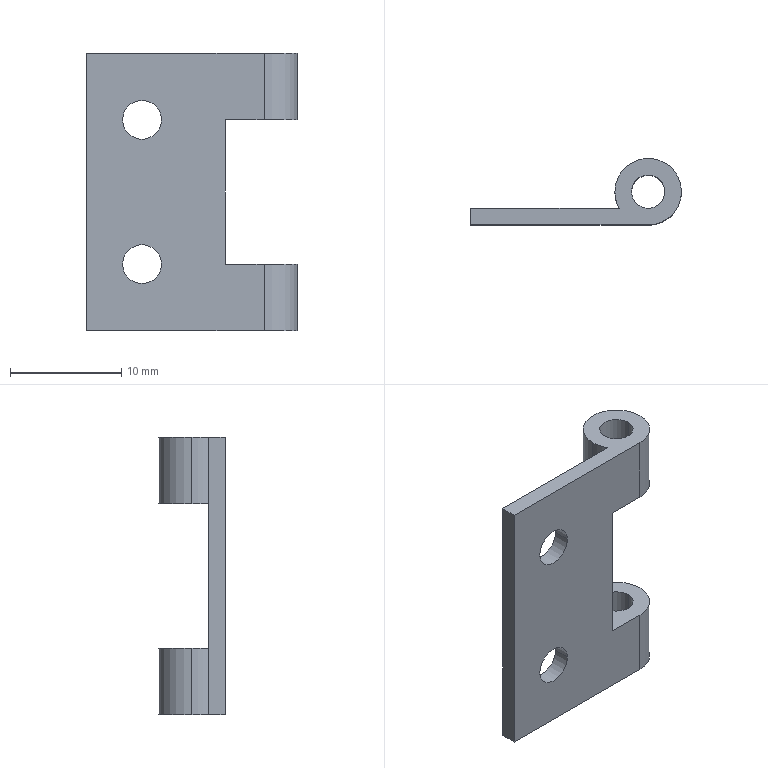Part | SolidWorks | features ICE 2, Extrusion 1 | 1 solid | 22 faces | box 19 x 6 x 25 mm | volume 724.19 mm3 | cylinder 14 | plane 8 | commonest cylinder face diameters 6 x6 3 x4 3.5 x4
STEP:
#1=CARTESIAN_POINT('',(-9.25,-3.,-6.5));
#2=VERTEX_POINT('',#1);
#3=CARTESIAN_POINT('',(-12.75,-3.,-6.5));
#4=VERTEX_POINT('',#3);
#5=CARTESIAN_POINT('',(-11.,-3.,-6.5));
#6=DIRECTION('',(0.,1.,0.));
#7=DIRECTION('',(-1.,0.,0.));
#8=AXIS2_PLACEMENT_3D('',#5,#6,#7);
#9=CIRCLE('',#8,1.75);
#10=EDGE_CURVE('',#2,#4,#9,.T.);
#11=ORIENTED_EDGE('',*,*,#10,.F.);
#12=CARTESIAN_POINT('',(-9.25,-1.5,-6.5));
#13=VERTEX_POINT('',#12);
#14=CARTESIAN_POINT('',(-9.25,-3.,-6.5));
#15=DIRECTION('',(0.,1.,0.));
#16=VECTOR('',#15,1000.);
#17=LINE('',#14,#16);
#18=EDGE_CURVE('',#2,#13,#17,.T.);
#19=ORIENTED_EDGE('',*,*,#18,.T.);
#20=CARTESIAN_POINT('',(-12.75,-1.5,-6.5));
#21=VERTEX_POINT('',#20);
#22=CARTESIAN_POINT('',(-11.,-1.5,-6.5));
#23=DIRECTION('',(0.,1.,0.));
#24=DIRECTION('',(-1.,0.,0.));
#25=AXIS2_PLACEMENT_3D('',#22,#23,#24);
#26=CIRCLE('',#25,1.75);
#27=EDGE_CURVE('',#13,#21,#26,.T.);
#28=ORIENTED_EDGE('',*,*,#27,.T.);
#29=CARTESIAN_POINT('',(-12.75,-3.,-6.5));
#30=DIRECTION('',(0.,1.,0.));
#31=VECTOR('',#30,1000.);
#32=LINE('',#29,#31);
#33=EDGE_CURVE('',#4,#21,#32,.T.);
#34=ORIENTED_EDGE('',*,*,#33,.F.);
#35=EDGE_LOOP('',(#11,#19,#28,#34));
#36=FACE_OUTER_BOUND('',#35,.T.);
#37=CARTESIAN_POINT('',(-11.,-3.,-6.5));
#38=DIRECTION('',(0.,1.,0.));
#39=DIRECTION('',(-1.,0.,0.));
#40=AXIS2_PLACEMENT_3D('',#37,#38,#39);
#41=CYLINDRICAL_SURFACE('',#40,1.75);
#42=ADVANCED_FACE('',(#36),#41,.F.);
#43=CARTESIAN_POINT('',(-9.25,-3.,6.5));
#44=VERTEX_POINT('',#43);
#45=CARTESIAN_POINT('',(-12.75,-3.,6.5));
#46=VERTEX_POINT('',#45);
#47=CARTESIAN_POINT('',(-11.,-3.,6.5));
#48=DIRECTION('',(0.,1.,0.));
#49=DIRECTION('',(1.,0.,0.));
#50=AXIS2_PLACEMENT_3D('',#47,#48,#49);
#51=CIRCLE('',#50,1.75);
#52=EDGE_CURVE('',#44,#46,#51,.T.);
#53=ORIENTED_EDGE('',*,*,#52,.F.);
#54=CARTESIAN_POINT('',(-9.25,-1.5,6.5));
#55=VERTEX_POINT('',#54);
#56=CARTESIAN_POINT('',(-9.25,-3.,6.5));
#57=DIRECTION('',(0.,1.,0.));
#58=VECTOR('',#57,1000.);
#59=LINE('',#56,#58);
#60=EDGE_CURVE('',#44,#55,#59,.T.);
#61=ORIENTED_EDGE('',*,*,#60,.T.);
#62=CARTESIAN_POINT('',(-12.75,-1.5,6.5));
#63=VERTEX_POINT('',#62);
#64=CARTESIAN_POINT('',(-11.,-1.5,6.5));
#65=DIRECTION('',(0.,1.,0.));
#66=DIRECTION('',(1.,0.,0.));
#67=AXIS2_PLACEMENT_3D('',#64,#65,#66);
#68=CIRCLE('',#67,1.75);
#69=EDGE_CURVE('',#55,#63,#68,.T.);
#70=ORIENTED_EDGE('',*,*,#69,.T.);
#71=CARTESIAN_POINT('',(-12.75,-3.,6.5));
#72=DIRECTION('',(0.,1.,0.));
#73=VECTOR('',#72,1000.);
#74=LINE('',#71,#73);
#75=EDGE_CURVE('',#46,#63,#74,.T.);
#76=ORIENTED_EDGE('',*,*,#75,.F.);
#77=EDGE_LOOP('',(#53,#61,#70,#76));
#78=FACE_OUTER_BOUND('',#77,.T.);
#79=CARTESIAN_POINT('',(-11.,-3.,6.5));
#80=DIRECTION('',(0.,1.,0.));
#81=DIRECTION('',(-1.,0.,0.));
#82=AXIS2_PLACEMENT_3D('',#79,#80,#81);
#83=CYLINDRICAL_SURFACE('',#82,1.75);
#84=ADVANCED_FACE('',(#78),#83,.F.);
#85=CARTESIAN_POINT('',(-1.5,0.,12.5));
#86=VERTEX_POINT('',#85);
#87=CARTESIAN_POINT('',(1.5,0.,12.5));
#88=VERTEX_POINT('',#87);
#89=CARTESIAN_POINT('',(0.,0.,12.5));
#90=DIRECTION('',(0.,0.,1.));
#91=DIRECTION('',(1.,0.,0.));
#92=AXIS2_PLACEMENT_3D('',#89,#90,#91);
#93=CIRCLE('',#92,1.5);
#94=EDGE_CURVE('',#86,#88,#93,.T.);
#95=ORIENTED_EDGE('',*,*,#94,.T.);
#96=CARTESIAN_POINT('',(1.5,0.,6.5));
#97=VERTEX_POINT('',#96);
#98=CARTESIAN_POINT('',(1.5,0.,12.5));
#99=DIRECTION('',(0.,0.,-1.));
#100=VECTOR('',#99,1000.);
#101=LINE('',#98,#100);
#102=EDGE_CURVE('',#88,#97,#101,.T.);
#103=ORIENTED_EDGE('',*,*,#102,.T.);
#104=CARTESIAN_POINT('',(-1.5,0.,6.5));
#105=VERTEX_POINT('',#104);
#106=CARTESIAN_POINT('',(0.,0.,6.5));
#107=DIRECTION('',(0.,0.,1.));
#108=DIRECTION('',(1.,0.,0.));
#109=AXIS2_PLACEMENT_3D('',#106,#107,#108);
#110=CIRCLE('',#109,1.5);
#111=EDGE_CURVE('',#105,#97,#110,.T.);
#112=ORIENTED_EDGE('',*,*,#111,.F.);
#113=CARTESIAN_POINT('',(-1.5,0.,12.5));
#114=DIRECTION('',(0.,0.,-1.));
#115=VECTOR('',#114,1000.);
#116=LINE('',#113,#115);
#117=EDGE_CURVE('',#86,#105,#116,.T.);
#118=ORIENTED_EDGE('',*,*,#117,.F.);
#119=EDGE_LOOP('',(#95,#103,#112,#118));
#120=FACE_OUTER_BOUND('',#119,.T.);
#121=CARTESIAN_POINT('',(0.,0.,12.5));
#122=DIRECTION('',(0.,0.,-1.));
#123=DIRECTION('',(-1.,0.,0.));
#124=AXIS2_PLACEMENT_3D('',#121,#122,#123);
#125=CYLINDRICAL_SURFACE('',#124,1.5);
#126=ADVANCED_FACE('',(#120),#125,.F.);
#127=CARTESIAN_POINT('',(3.,0.,12.5));
#128=VERTEX_POINT('',#127);
#129=CARTESIAN_POINT('',(-3.,0.,12.5));
#130=VERTEX_POINT('',#129);
#131=CARTESIAN_POINT('',(0.,0.,12.5));
#132=DIRECTION('',(0.,0.,1.));
#133=DIRECTION('',(1.,0.,0.));
#134=AXIS2_PLACEMENT_3D('',#131,#132,#133);
#135=CIRCLE('',#134,3.);
#136=EDGE_CURVE('',#128,#130,#135,.T.);
#137=ORIENTED_EDGE('',*,*,#136,.F.);
#138=CARTESIAN_POINT('',(3.,0.,6.5));
#139=VERTEX_POINT('',#138);
#140=CARTESIAN_POINT('',(3.,0.,12.5));
#141=DIRECTION('',(0.,0.,-1.));
#142=VECTOR('',#141,1000.);
#143=LINE('',#140,#142);
#144=EDGE_CURVE('',#128,#139,#143,.T.);
#145=ORIENTED_EDGE('',*,*,#144,.T.);
#146=CARTESIAN_POINT('',(-3.,0.,6.5));
#147=VERTEX_POINT('',#146);
#148=CARTESIAN_POINT('',(0.,0.,6.5));
#149=DIRECTION('',(0.,0.,1.));
#150=DIRECTION('',(1.,0.,0.));
#151=AXIS2_PLACEMENT_3D('',#148,#149,#150);
#152=CIRCLE('',#151,3.);
#153=EDGE_CURVE('',#139,#147,#152,.T.);
#154=ORIENTED_EDGE('',*,*,#153,.T.);
#155=CARTESIAN_POINT('',(-3.,0.,12.5));
#156=DIRECTION('',(0.,0.,-1.));
#157=VECTOR('',#156,1000.);
#158=LINE('',#155,#157);
#159=EDGE_CURVE('',#130,#147,#158,.T.);
#160=ORIENTED_EDGE('',*,*,#159,.F.);
#161=EDGE_LOOP('',(#137,#145,#154,#160));
#162=FACE_OUTER_BOUND('',#161,.T.);
#163=CARTESIAN_POINT('',(0.,0.,12.5));
#164=DIRECTION('',(0.,0.,-1.));
#165=DIRECTION('',(-1.,0.,0.));
#166=AXIS2_PLACEMENT_3D('',#163,#164,#165);
#167=CYLINDRICAL_SURFACE('',#166,3.);
#168=ADVANCED_FACE('',(#162),#167,.T.);
#169=CARTESIAN_POINT('',(-2.598,-1.5,12.5));
#170=VERTEX_POINT('',#169);
#171=CARTESIAN_POINT('',(0.,0.,12.5));
#172=DIRECTION('',(0.,0.,1.));
#173=DIRECTION('',(1.,0.,0.));
#174=AXIS2_PLACEMENT_3D('',#171,#172,#173);
#175=CIRCLE('',#174,3.);
#176=EDGE_CURVE('',#130,#170,#175,.T.);
#177=ORIENTED_EDGE('',*,*,#176,.F.);
#178=ORIENTED_EDGE('',*,*,#159,.T.);
#179=CARTESIAN_POINT('',(-2.598,-1.5,6.5));
#180=VERTEX_POINT('',#179);
#181=CARTESIAN_POINT('',(0.,0.,6.5));
#182=DIRECTION('',(0.,0.,1.));
#183=DIRECTION('',(1.,0.,0.));
#184=AXIS2_PLACEMENT_3D('',#181,#182,#183);
#185=CIRCLE('',#184,3.);
#186=EDGE_CURVE('',#147,#180,#185,.T.);
#187=ORIENTED_EDGE('',*,*,#186,.T.);
#188=CARTESIAN_POINT('',(-2.598,-1.5,12.5));
#189=DIRECTION('',(0.,0.,-1.));
#190=VECTOR('',#189,1000.);
#191=LINE('',#188,#190);
#192=EDGE_CURVE('',#170,#180,#191,.T.);
#193=ORIENTED_EDGE('',*,*,#192,.F.);
#194=EDGE_LOOP('',(#177,#178,#187,#193));
#195=FACE_OUTER_BOUND('',#194,.T.);
#196=CARTESIAN_POINT('',(0.,0.,12.5));
#197=DIRECTION('',(0.,0.,-1.));
#198=DIRECTION('',(-1.,0.,0.));
#199=AXIS2_PLACEMENT_3D('',#196,#197,#198);
#200=CYLINDRICAL_SURFACE('',#199,3.);
#201=ADVANCED_FACE('',(#195),#200,.T.);
#202=CARTESIAN_POINT('',(-1.5,0.,-6.5));
#203=VERTEX_POINT('',#202);
#204=CARTESIAN_POINT('',(1.5,0.,-6.5));
#205=VERTEX_POINT('',#204);
#206=CARTESIAN_POINT('',(0.,0.,-6.5));
#207=DIRECTION('',(0.,0.,1.));
#208=DIRECTION('',(1.,0.,0.));
#209=AXIS2_PLACEMENT_3D('',#206,#207,#208);
#210=CIRCLE('',#209,1.5);
#211=EDGE_CURVE('',#203,#205,#210,.T.);
#212=ORIENTED_EDGE('',*,*,#211,.T.);
#213=CARTESIAN_POINT('',(1.5,0.,-12.5));
#214=VERTEX_POINT('',#213);
#215=CARTESIAN_POINT('',(1.5,0.,12.5));
#216=DIRECTION('',(0.,0.,-1.));
#217=VECTOR('',#216,1000.);
#218=LINE('',#215,#217);
#219=EDGE_CURVE('',#205,#214,#218,.T.);
#220=ORIENTED_EDGE('',*,*,#219,.T.);
#221=CARTESIAN_POINT('',(-1.5,0.,-12.5));
#222=VERTEX_POINT('',#221);
#223=CARTESIAN_POINT('',(0.,0.,-12.5));
#224=DIRECTION('',(0.,0.,1.));
#225=DIRECTION('',(1.,0.,0.));
#226=AXIS2_PLACEMENT_3D('',#223,#224,#225);
#227=CIRCLE('',#226,1.5);
#228=EDGE_CURVE('',#222,#214,#227,.T.);
#229=ORIENTED_EDGE('',*,*,#228,.F.);
#230=CARTESIAN_POINT('',(-1.5,0.,12.5));
#231=DIRECTION('',(0.,0.,-1.));
#232=VECTOR('',#231,1000.);
#233=LINE('',#230,#232);
#234=EDGE_CURVE('',#203,#222,#233,.T.);
#235=ORIENTED_EDGE('',*,*,#234,.F.);
#236=EDGE_LOOP('',(#212,#220,#229,#235));
#237=FACE_OUTER_BOUND('',#236,.T.);
#238=CARTESIAN_POINT('',(0.,0.,12.5));
#239=DIRECTION('',(0.,0.,-1.));
#240=DIRECTION('',(-1.,0.,0.));
#241=AXIS2_PLACEMENT_3D('',#238,#239,#240);
#242=CYLINDRICAL_SURFACE('',#241,1.5);
#243=ADVANCED_FACE('',(#237),#242,.F.);
#244=CARTESIAN_POINT('',(3.,0.,-6.5));
#245=VERTEX_POINT('',#244);
#246=CARTESIAN_POINT('',(-3.,0.,-6.5));
#247=VERTEX_POINT('',#246);
#248=CARTESIAN_POINT('',(0.,0.,-6.5));
#249=DIRECTION('',(0.,0.,1.));
#250=DIRECTION('',(1.,0.,0.));
#251=AXIS2_PLACEMENT_3D('',#248,#249,#250);
#252=CIRCLE('',#251,3.);
#253=EDGE_CURVE('',#245,#247,#252,.T.);
#254=ORIENTED_EDGE('',*,*,#253,.F.);
#255=CARTESIAN_POINT('',(3.,0.,-12.5));
#256=VERTEX_POINT('',#255);
#257=CARTESIAN_POINT('',(3.,0.,12.5));
#258=DIRECTION('',(0.,0.,-1.));
#259=VECTOR('',#258,1000.);
#260=LINE('',#257,#259);
#261=EDGE_CURVE('',#245,#256,#260,.T.);
#262=ORIENTED_EDGE('',*,*,#261,.T.);
#263=CARTESIAN_POINT('',(-3.,0.,-12.5));
#264=VERTEX_POINT('',#263);
#265=CARTESIAN_POINT('',(0.,0.,-12.5));
#266=DIRECTION('',(0.,0.,1.));
#267=DIRECTION('',(1.,0.,0.));
#268=AXIS2_PLACEMENT_3D('',#265,#266,#267);
#269=CIRCLE('',#268,3.);
#270=EDGE_CURVE('',#256,#264,#269,.T.);
#271=ORIENTED_EDGE('',*,*,#270,.T.);
#272=CARTESIAN_POINT('',(-3.,0.,12.5));
#273=DIRECTION('',(0.,0.,-1.));
#274=VECTOR('',#273,1000.);
#275=LINE('',#272,#274);
#276=EDGE_CURVE('',#247,#264,#275,.T.);
#277=ORIENTED_EDGE('',*,*,#276,.F.);
#278=EDGE_LOOP('',(#254,#262,#271,#277));
#279=FACE_OUTER_BOUND('',#278,.T.);
#280=CARTESIAN_POINT('',(0.,0.,12.5));
#281=DIRECTION('',(0.,0.,-1.));
#282=DIRECTION('',(-1.,0.,0.));
#283=AXIS2_PLACEMENT_3D('',#280,#281,#282);
#284=CYLINDRICAL_SURFACE('',#283,3.);
#285=ADVANCED_FACE('',(#279),#284,.T.);
#286=CARTESIAN_POINT('',(-2.598,-1.5,-6.5));
#287=VERTEX_POINT('',#286);
#288=CARTESIAN_POINT('',(0.,0.,-6.5));
#289=DIRECTION('',(0.,0.,1.));
#290=DIRECTION('',(1.,0.,0.));
#291=AXIS2_PLACEMENT_3D('',#288,#289,#290);
#292=CIRCLE('',#291,3.);
#293=EDGE_CURVE('',#247,#287,#292,.T.);
#294=ORIENTED_EDGE('',*,*,#293,.F.);
#295=ORIENTED_EDGE('',*,*,#276,.T.);
#296=CARTESIAN_POINT('',(-2.598,-1.5,-12.5));
#297=VERTEX_POINT('',#296);
#298=CARTESIAN_POINT('',(0.,0.,-12.5));
#299=DIRECTION('',(0.,0.,1.));
#300=DIRECTION('',(1.,0.,0.));
#301=AXIS2_PLACEMENT_3D('',#298,#299,#300);
#302=CIRCLE('',#301,3.);
#303=EDGE_CURVE('',#264,#297,#302,.T.);
#304=ORIENTED_EDGE('',*,*,#303,.T.);
#305=CARTESIAN_POINT('',(-2.598,-1.5,12.5));
#306=DIRECTION('',(0.,0.,-1.));
#307=VECTOR('',#306,1000.);
#308=LINE('',#305,#307);
#309=EDGE_CURVE('',#287,#297,#308,.T.);
#310=ORIENTED_EDGE('',*,*,#309,.F.);
#311=EDGE_LOOP('',(#294,#295,#304,#310));
#312=FACE_OUTER_BOUND('',#311,.T.);
#313=CARTESIAN_POINT('',(0.,0.,12.5));
#314=DIRECTION('',(0.,0.,-1.));
#315=DIRECTION('',(-1.,0.,0.));
#316=AXIS2_PLACEMENT_3D('',#313,#314,#315);
#317=CYLINDRICAL_SURFACE('',#316,3.);
#318=ADVANCED_FACE('',(#312),#317,.T.);
#319=CARTESIAN_POINT('',(-11.,-3.,-6.5));
#320=DIRECTION('',(0.,1.,0.));
#321=DIRECTION('',(-1.,0.,0.));
#322=AXIS2_PLACEMENT_3D('',#319,#320,#321);
#323=CIRCLE('',#322,1.75);
#324=EDGE_CURVE('',#4,#2,#323,.T.);
#325=ORIENTED_EDGE('',*,*,#324,.T.);
#326=ORIENTED_EDGE('',*,*,#10,.T.);
#327=EDGE_LOOP('',(#325,#326));
#328=FACE_BOUND('',#327,.T.);
#329=CARTESIAN_POINT('',(-11.,-3.,6.5));
#330=DIRECTION('',(0.,1.,0.));
#331=DIRECTION('',(1.,0.,0.));
#332=AXIS2_PLACEMENT_3D('',#329,#330,#331);
#333=CIRCLE('',#332,1.75);
#334=EDGE_CURVE('',#46,#44,#333,.T.);
#335=ORIENTED_EDGE('',*,*,#334,.T.);
#336=ORIENTED_EDGE('',*,*,#52,.T.);
#337=EDGE_LOOP('',(#335,#336));
#338=FACE_BOUND('',#337,.T.);
#339=CARTESIAN_POINT('',(0.,-3.,-6.5));
#340=VERTEX_POINT('',#339);
#341=CARTESIAN_POINT('',(0.,-3.,-12.5));
#342=VERTEX_POINT('',#341);
#343=CARTESIAN_POINT('',(0.,-3.,12.5));
#344=DIRECTION('',(0.,0.,-1.));
#345=VECTOR('',#344,1000.);
#346=LINE('',#343,#345);
#347=EDGE_CURVE('',#340,#342,#346,.T.);
#348=ORIENTED_EDGE('',*,*,#347,.F.);
#349=CARTESIAN_POINT('',(-3.5,-3.,-6.5));
#350=VERTEX_POINT('',#349);
#351=CARTESIAN_POINT('',(-3.5,-3.,-6.5));
#352=DIRECTION('',(1.,0.,0.));
#353=VECTOR('',#352,1000.);
#354=LINE('',#351,#353);
#355=EDGE_CURVE('',#350,#340,#354,.T.);
#356=ORIENTED_EDGE('',*,*,#355,.F.);
#357=CARTESIAN_POINT('',(-3.5,-3.,6.5));
#358=VERTEX_POINT('',#357);
#359=CARTESIAN_POINT('',(-3.5,-3.,-6.5));
#360=DIRECTION('',(0.,0.,1.));
#361=VECTOR('',#360,1000.);
#362=LINE('',#359,#361);
#363=EDGE_CURVE('',#350,#358,#362,.T.);
#364=ORIENTED_EDGE('',*,*,#363,.T.);
#365=CARTESIAN_POINT('',(0.,-3.,6.5));
#366=VERTEX_POINT('',#365);
#367=CARTESIAN_POINT('',(-3.5,-3.,6.5));
#368=DIRECTION('',(1.,0.,0.));
#369=VECTOR('',#368,1000.);
#370=LINE('',#367,#369);
#371=EDGE_CURVE('',#358,#366,#370,.T.);
#372=ORIENTED_EDGE('',*,*,#371,.T.);
#373=CARTESIAN_POINT('',(0.,-3.,12.5));
#374=VERTEX_POINT('',#373);
#375=CARTESIAN_POINT('',(0.,-3.,12.5));
#376=DIRECTION('',(0.,0.,-1.));
#377=VECTOR('',#376,1000.);
#378=LINE('',#375,#377);
#379=EDGE_CURVE('',#374,#366,#378,.T.);
#380=ORIENTED_EDGE('',*,*,#379,.F.);
#381=CARTESIAN_POINT('',(-16.,-3.,12.5));
#382=VERTEX_POINT('',#381);
#383=CARTESIAN_POINT('',(-16.,-3.,12.5));
#384=DIRECTION('',(1.,0.,0.));
#385=VECTOR('',#384,1000.);
#386=LINE('',#383,#385);
#387=EDGE_CURVE('',#382,#374,#386,.T.);
#388=ORIENTED_EDGE('',*,*,#387,.F.);
#389=CARTESIAN_POINT('',(-16.,-3.,-12.5));
#390=VERTEX_POINT('',#389);
#391=CARTESIAN_POINT('',(-16.,-3.,12.5));
#392=DIRECTION('',(0.,0.,-1.));
#393=VECTOR('',#392,1000.);
#394=LINE('',#391,#393);
#395=EDGE_CURVE('',#382,#390,#394,.T.);
#396=ORIENTED_EDGE('',*,*,#395,.T.);
#397=CARTESIAN_POINT('',(-16.,-3.,-12.5));
#398=DIRECTION('',(1.,0.,0.));
#399=VECTOR('',#398,1000.);
#400=LINE('',#397,#399);
#401=EDGE_CURVE('',#390,#342,#400,.T.);
#402=ORIENTED_EDGE('',*,*,#401,.T.);
#403=EDGE_LOOP('',(#348,#356,#364,#372,#380,#388,#396,#402));
#404=FACE_OUTER_BOUND('',#403,.T.);
#405=CARTESIAN_POINT('',(-16.,-3.,12.5));
#406=DIRECTION('',(0.,1.,0.));
#407=DIRECTION('',(-1.,0.,0.));
#408=AXIS2_PLACEMENT_3D('',#405,#406,#407);
#409=PLANE('',#408);
#410=ADVANCED_FACE('',(#328,#338,#404),#409,.F.);
#411=ORIENTED_EDGE('',*,*,#261,.F.);
#412=CARTESIAN_POINT('',(0.,0.,-6.5));
#413=DIRECTION('',(0.,0.,1.));
#414=DIRECTION('',(1.,0.,0.));
#415=AXIS2_PLACEMENT_3D('',#412,#413,#414);
#416=CIRCLE('',#415,3.);
#417=EDGE_CURVE('',#340,#245,#416,.T.);
#418=ORIENTED_EDGE('',*,*,#417,.F.);
#419=ORIENTED_EDGE('',*,*,#347,.T.);
#420=CARTESIAN_POINT('',(0.,0.,-12.5));
#421=DIRECTION('',(0.,0.,1.));
#422=DIRECTION('',(1.,0.,0.));
#423=AXIS2_PLACEMENT_3D('',#420,#421,#422);
#424=CIRCLE('',#423,3.);
#425=EDGE_CURVE('',#342,#256,#424,.T.);
#426=ORIENTED_EDGE('',*,*,#425,.T.);
#427=EDGE_LOOP('',(#411,#418,#419,#426));
#428=FACE_OUTER_BOUND('',#427,.T.);
#429=CARTESIAN_POINT('',(0.,0.,12.5));
#430=DIRECTION('',(0.,0.,-1.));
#431=DIRECTION('',(-1.,0.,0.));
#432=AXIS2_PLACEMENT_3D('',#429,#430,#431);
#433=CYLINDRICAL_SURFACE('',#432,3.);
#434=ADVANCED_FACE('',(#428),#433,.T.);
#435=CARTESIAN_POINT('',(-11.,-1.5,-6.5));
#436=DIRECTION('',(0.,1.,0.));
#437=DIRECTION('',(-1.,0.,0.));
#438=AXIS2_PLACEMENT_3D('',#435,#436,#437);
#439=CIRCLE('',#438,1.75);
#440=EDGE_CURVE('',#21,#13,#439,.T.);
#441=ORIENTED_EDGE('',*,*,#440,.F.);
#442=ORIENTED_EDGE('',*,*,#27,.F.);
#443=EDGE_LOOP('',(#441,#442));
#444=FACE_BOUND('',#443,.T.);
#445=CARTESIAN_POINT('',(-11.,-1.5,6.5));
#446=DIRECTION('',(0.,1.,0.));
#447=DIRECTION('',(1.,0.,0.));
#448=AXIS2_PLACEMENT_3D('',#445,#446,#447);
#449=CIRCLE('',#448,1.75);
#450=EDGE_CURVE('',#63,#55,#449,.T.);
#451=ORIENTED_EDGE('',*,*,#450,.F.);
#452=ORIENTED_EDGE('',*,*,#69,.F.);
#453=EDGE_LOOP('',(#451,#452));
#454=FACE_BOUND('',#453,.T.);
#455=CARTESIAN_POINT('',(-3.5,-1.5,-6.5));
#456=VERTEX_POINT('',#455);
#457=CARTESIAN_POINT('',(-2.598,-1.5,-6.5));
#458=DIRECTION('',(-1.,0.,0.));
#459=VECTOR('',#458,1000.);
#460=LINE('',#457,#459);
#461=EDGE_CURVE('',#287,#456,#460,.T.);
#462=ORIENTED_EDGE('',*,*,#461,.F.);
#463=ORIENTED_EDGE('',*,*,#309,.T.);
#464=CARTESIAN_POINT('',(-16.,-1.5,-12.5));
#465=VERTEX_POINT('',#464);
#466=CARTESIAN_POINT('',(-2.598,-1.5,-12.5));
#467=DIRECTION('',(-1.,0.,0.));
#468=VECTOR('',#467,1000.);
#469=LINE('',#466,#468);
#470=EDGE_CURVE('',#297,#465,#469,.T.);
#471=ORIENTED_EDGE('',*,*,#470,.T.);
#472=CARTESIAN_POINT('',(-16.,-1.5,12.5));
#473=VERTEX_POINT('',#472);
#474=CARTESIAN_POINT('',(-16.,-1.5,12.5));
#475=DIRECTION('',(0.,0.,-1.));
#476=VECTOR('',#475,1000.);
#477=LINE('',#474,#476);
#478=EDGE_CURVE('',#473,#465,#477,.T.);
#479=ORIENTED_EDGE('',*,*,#478,.F.);
#480=CARTESIAN_POINT('',(-2.598,-1.5,12.5));
#481=DIRECTION('',(-1.,0.,0.));
#482=VECTOR('',#481,1000.);
#483=LINE('',#480,#482);
#484=EDGE_CURVE('',#170,#473,#483,.T.);
#485=ORIENTED_EDGE('',*,*,#484,.F.);
#486=ORIENTED_EDGE('',*,*,#192,.T.);
#487=CARTESIAN_POINT('',(-3.5,-1.5,6.5));
#488=VERTEX_POINT('',#487);
#489=CARTESIAN_POINT('',(-2.598,-1.5,6.5));
#490=DIRECTION('',(-1.,0.,0.));
#491=VECTOR('',#490,1000.);
#492=LINE('',#489,#491);
#493=EDGE_CURVE('',#180,#488,#492,.T.);
#494=ORIENTED_EDGE('',*,*,#493,.T.);
#495=CARTESIAN_POINT('',(-3.5,-1.5,12.5));
#496=DIRECTION('',(0.,0.,-1.));
#497=VECTOR('',#496,1000.);
#498=LINE('',#495,#497);
#499=EDGE_CURVE('',#488,#456,#498,.T.);
#500=ORIENTED_EDGE('',*,*,#499,.T.);
#501=EDGE_LOOP('',(#462,#463,#471,#479,#485,#486,#494,#500));
#502=FACE_OUTER_BOUND('',#501,.T.);
#503=CARTESIAN_POINT('',(-2.598,-1.5,12.5));
#504=DIRECTION('',(0.,-1.,0.));
#505=DIRECTION('',(1.,0.,0.));
#506=AXIS2_PLACEMENT_3D('',#503,#504,#505);
#507=PLANE('',#506);
#508=ADVANCED_FACE('',(#444,#454,#502),#507,.F.);
#509=ORIENTED_EDGE('',*,*,#219,.F.);
#510=CARTESIAN_POINT('',(0.,0.,-6.5));
#511=DIRECTION('',(0.,0.,1.));
#512=DIRECTION('',(1.,0.,0.));
#513=AXIS2_PLACEMENT_3D('',#510,#511,#512);
#514=CIRCLE('',#513,1.5);
#515=EDGE_CURVE('',#205,#203,#514,.T.);
#516=ORIENTED_EDGE('',*,*,#515,.T.);
#517=ORIENTED_EDGE('',*,*,#234,.T.);
#518=CARTESIAN_POINT('',(0.,0.,-12.5));
#519=DIRECTION('',(0.,0.,1.));
#520=DIRECTION('',(1.,0.,0.));
#521=AXIS2_PLACEMENT_3D('',#518,#519,#520);
#522=CIRCLE('',#521,1.5);
#523=EDGE_CURVE('',#214,#222,#522,.T.);
#524=ORIENTED_EDGE('',*,*,#523,.F.);
#525=EDGE_LOOP('',(#509,#516,#517,#524));
#526=FACE_OUTER_BOUND('',#525,.T.);
#527=CARTESIAN_POINT('',(0.,0.,12.5));
#528=DIRECTION('',(0.,0.,-1.));
#529=DIRECTION('',(-1.,0.,0.));
#530=AXIS2_PLACEMENT_3D('',#527,#528,#529);
#531=CYLINDRICAL_SURFACE('',#530,1.5);
#532=ADVANCED_FACE('',(#526),#531,.F.);
#533=CARTESIAN_POINT('',(-16.,-1.5,12.5));
#534=DIRECTION('',(0.,-1.,0.));
#535=VECTOR('',#534,1000.);
#536=LINE('',#533,#535);
#537=EDGE_CURVE('',#473,#382,#536,.T.);
#538=ORIENTED_EDGE('',*,*,#537,.T.);
#539=ORIENTED_EDGE('',*,*,#387,.T.);
#540=CARTESIAN_POINT('',(0.,0.,12.5));
#541=DIRECTION('',(0.,0.,1.));
#542=DIRECTION('',(1.,0.,0.));
#543=AXIS2_PLACEMENT_3D('',#540,#541,#542);
#544=CIRCLE('',#543,3.);
#545=EDGE_CURVE('',#374,#128,#544,.T.);
#546=ORIENTED_EDGE('',*,*,#545,.T.);
#547=ORIENTED_EDGE('',*,*,#136,.T.);
#548=ORIENTED_EDGE('',*,*,#176,.T.);
#549=ORIENTED_EDGE('',*,*,#484,.T.);
#550=EDGE_LOOP('',(#538,#539,#546,#547,#548,#549));
#551=FACE_OUTER_BOUND('',#550,.T.);
#552=ORIENTED_EDGE('',*,*,#94,.F.);
#553=CARTESIAN_POINT('',(0.,0.,12.5));
#554=DIRECTION('',(0.,0.,1.));
#555=DIRECTION('',(1.,0.,0.));
#556=AXIS2_PLACEMENT_3D('',#553,#554,#555);
#557=CIRCLE('',#556,1.5);
#558=EDGE_CURVE('',#88,#86,#557,.T.);
#559=ORIENTED_EDGE('',*,*,#558,.F.);
#560=EDGE_LOOP('',(#552,#559));
#561=FACE_BOUND('',#560,.T.);
#562=CARTESIAN_POINT('',(0.,0.,12.5));
#563=DIRECTION('',(0.,0.,1.));
#564=DIRECTION('',(1.,0.,0.));
#565=AXIS2_PLACEMENT_3D('',#562,#563,#564);
#566=PLANE('',#565);
#567=ADVANCED_FACE('',(#551,#561),#566,.T.);
#568=CARTESIAN_POINT('',(-16.,-1.5,-12.5));
#569=DIRECTION('',(0.,-1.,0.));
#570=VECTOR('',#569,1000.);
#571=LINE('',#568,#570);
#572=EDGE_CURVE('',#465,#390,#571,.T.);
#573=ORIENTED_EDGE('',*,*,#572,.F.);
#574=ORIENTED_EDGE('',*,*,#470,.F.);
#575=ORIENTED_EDGE('',*,*,#303,.F.);
#576=ORIENTED_EDGE('',*,*,#270,.F.);
#577=ORIENTED_EDGE('',*,*,#425,.F.);
#578=ORIENTED_EDGE('',*,*,#401,.F.);
#579=EDGE_LOOP('',(#573,#574,#575,#576,#577,#578));
#580=FACE_OUTER_BOUND('',#579,.T.);
#581=ORIENTED_EDGE('',*,*,#228,.T.);
#582=ORIENTED_EDGE('',*,*,#523,.T.);
#583=EDGE_LOOP('',(#581,#582));
#584=FACE_BOUND('',#583,.T.);
#585=CARTESIAN_POINT('',(0.,0.,-12.5));
#586=DIRECTION('',(0.,0.,1.));
#587=DIRECTION('',(1.,0.,0.));
#588=AXIS2_PLACEMENT_3D('',#585,#586,#587);
#589=PLANE('',#588);
#590=ADVANCED_FACE('',(#580,#584),#589,.F.);
#591=ORIENTED_EDGE('',*,*,#572,.T.);
#592=ORIENTED_EDGE('',*,*,#395,.F.);
#593=ORIENTED_EDGE('',*,*,#537,.F.);
#594=ORIENTED_EDGE('',*,*,#478,.T.);
#595=EDGE_LOOP('',(#591,#592,#593,#594));
#596=FACE_OUTER_BOUND('',#595,.T.);
#597=CARTESIAN_POINT('',(-16.,-1.5,12.5));
#598=DIRECTION('',(1.,0.,0.));
#599=DIRECTION('',(0.,0.,-1.));
#600=AXIS2_PLACEMENT_3D('',#597,#598,#599);
#601=PLANE('',#600);
#602=ADVANCED_FACE('',(#596),#601,.F.);
#603=ORIENTED_EDGE('',*,*,#144,.F.);
#604=ORIENTED_EDGE('',*,*,#545,.F.);
#605=ORIENTED_EDGE('',*,*,#379,.T.);
#606=CARTESIAN_POINT('',(0.,0.,6.5));
#607=DIRECTION('',(0.,0.,1.));
#608=DIRECTION('',(1.,0.,0.));
#609=AXIS2_PLACEMENT_3D('',#606,#607,#608);
#610=CIRCLE('',#609,3.);
#611=EDGE_CURVE('',#366,#139,#610,.T.);
#612=ORIENTED_EDGE('',*,*,#611,.T.);
#613=EDGE_LOOP('',(#603,#604,#605,#612));
#614=FACE_OUTER_BOUND('',#613,.T.);
#615=CARTESIAN_POINT('',(0.,0.,12.5));
#616=DIRECTION('',(0.,0.,-1.));
#617=DIRECTION('',(-1.,0.,0.));
#618=AXIS2_PLACEMENT_3D('',#615,#616,#617);
#619=CYLINDRICAL_SURFACE('',#618,3.);
#620=ADVANCED_FACE('',(#614),#619,.T.);
#621=ORIENTED_EDGE('',*,*,#102,.F.);
#622=ORIENTED_EDGE('',*,*,#558,.T.);
#623=ORIENTED_EDGE('',*,*,#117,.T.);
#624=CARTESIAN_POINT('',(0.,0.,6.5));
#625=DIRECTION('',(0.,0.,1.));
#626=DIRECTION('',(1.,0.,0.));
#627=AXIS2_PLACEMENT_3D('',#624,#625,#626);
#628=CIRCLE('',#627,1.5);
#629=EDGE_CURVE('',#97,#105,#628,.T.);
#630=ORIENTED_EDGE('',*,*,#629,.F.);
#631=EDGE_LOOP('',(#621,#622,#623,#630));
#632=FACE_OUTER_BOUND('',#631,.T.);
#633=CARTESIAN_POINT('',(0.,0.,12.5));
#634=DIRECTION('',(0.,0.,-1.));
#635=DIRECTION('',(-1.,0.,0.));
#636=AXIS2_PLACEMENT_3D('',#633,#634,#635);
#637=CYLINDRICAL_SURFACE('',#636,1.5);
#638=ADVANCED_FACE('',(#632),#637,.F.);
#639=CARTESIAN_POINT('',(-3.5,0.,6.5));
#640=DIRECTION('',(0.,-1.,0.));
#641=VECTOR('',#640,1000.);
#642=LINE('',#639,#641);
#643=EDGE_CURVE('',#488,#358,#642,.T.);
#644=ORIENTED_EDGE('',*,*,#643,.T.);
#645=ORIENTED_EDGE('',*,*,#363,.F.);
#646=CARTESIAN_POINT('',(-3.5,0.,-6.5));
#647=DIRECTION('',(0.,-1.,0.));
#648=VECTOR('',#647,1000.);
#649=LINE('',#646,#648);
#650=EDGE_CURVE('',#456,#350,#649,.T.);
#651=ORIENTED_EDGE('',*,*,#650,.F.);
#652=ORIENTED_EDGE('',*,*,#499,.F.);
#653=EDGE_LOOP('',(#644,#645,#651,#652));
#654=FACE_OUTER_BOUND('',#653,.T.);
#655=CARTESIAN_POINT('',(-3.5,0.,-6.5));
#656=DIRECTION('',(-1.,0.,0.));
#657=DIRECTION('',(0.,-1.,0.));
#658=AXIS2_PLACEMENT_3D('',#655,#656,#657);
#659=PLANE('',#658);
#660=ADVANCED_FACE('',(#654),#659,.F.);
#661=ORIENTED_EDGE('',*,*,#211,.F.);
#662=ORIENTED_EDGE('',*,*,#515,.F.);
#663=EDGE_LOOP('',(#661,#662));
#664=FACE_BOUND('',#663,.T.);
#665=ORIENTED_EDGE('',*,*,#355,.T.);
#666=ORIENTED_EDGE('',*,*,#417,.T.);
#667=ORIENTED_EDGE('',*,*,#253,.T.);
#668=ORIENTED_EDGE('',*,*,#293,.T.);
#669=ORIENTED_EDGE('',*,*,#461,.T.);
#670=ORIENTED_EDGE('',*,*,#650,.T.);
#671=EDGE_LOOP('',(#665,#666,#667,#668,#669,#670));
#672=FACE_OUTER_BOUND('',#671,.T.);
#673=CARTESIAN_POINT('',(0.,0.,-6.5));
#674=DIRECTION('',(0.,0.,1.));
#675=DIRECTION('',(1.,0.,0.));
#676=AXIS2_PLACEMENT_3D('',#673,#674,#675);
#677=PLANE('',#676);
#678=ADVANCED_FACE('',(#664,#672),#677,.T.);
#679=ORIENTED_EDGE('',*,*,#111,.T.);
#680=ORIENTED_EDGE('',*,*,#629,.T.);
#681=EDGE_LOOP('',(#679,#680));
#682=FACE_BOUND('',#681,.T.);
#683=ORIENTED_EDGE('',*,*,#371,.F.);
#684=ORIENTED_EDGE('',*,*,#643,.F.);
#685=ORIENTED_EDGE('',*,*,#493,.F.);
#686=ORIENTED_EDGE('',*,*,#186,.F.);
#687=ORIENTED_EDGE('',*,*,#153,.F.);
#688=ORIENTED_EDGE('',*,*,#611,.F.);
#689=EDGE_LOOP('',(#683,#684,#685,#686,#687,#688));
#690=FACE_OUTER_BOUND('',#689,.T.);
#691=CARTESIAN_POINT('',(0.,0.,6.5));
#692=DIRECTION('',(0.,0.,1.));
#693=DIRECTION('',(1.,0.,0.));
#694=AXIS2_PLACEMENT_3D('',#691,#692,#693);
#695=PLANE('',#694);
#696=ADVANCED_FACE('',(#682,#690),#695,.F.);
#697=ORIENTED_EDGE('',*,*,#60,.F.);
#698=ORIENTED_EDGE('',*,*,#334,.F.);
#699=ORIENTED_EDGE('',*,*,#75,.T.);
#700=ORIENTED_EDGE('',*,*,#450,.T.);
#701=EDGE_LOOP('',(#697,#698,#699,#700));
#702=FACE_OUTER_BOUND('',#701,.T.);
#703=CARTESIAN_POINT('',(-11.,-3.,6.5));
#704=DIRECTION('',(0.,1.,0.));
#705=DIRECTION('',(-1.,0.,0.));
#706=AXIS2_PLACEMENT_3D('',#703,#704,#705);
#707=CYLINDRICAL_SURFACE('',#706,1.75);
#708=ADVANCED_FACE('',(#702),#707,.F.);
#709=ORIENTED_EDGE('',*,*,#18,.F.);
#710=ORIENTED_EDGE('',*,*,#324,.F.);
#711=ORIENTED_EDGE('',*,*,#33,.T.);
#712=ORIENTED_EDGE('',*,*,#440,.T.);
#713=EDGE_LOOP('',(#709,#710,#711,#712));
#714=FACE_OUTER_BOUND('',#713,.T.);
#715=CARTESIAN_POINT('',(-11.,-3.,-6.5));
#716=DIRECTION('',(0.,1.,0.));
#717=DIRECTION('',(-1.,0.,0.));
#718=AXIS2_PLACEMENT_3D('',#715,#716,#717);
#719=CYLINDRICAL_SURFACE('',#718,1.75);
#720=ADVANCED_FACE('',(#714),#719,.F.);
#721=CLOSED_SHELL('',(#42,#84,#126,#168,#201,#243,#285,#318,#410,#434,#508,#532,#567,#590,#602,#620,#638,#660,#678,#696,#708,#720));
#722=MANIFOLD_SOLID_BREP('',#721);
#723=CARTESIAN_POINT('',(0.,0.,0.));
#724=DIRECTION('',(0.,0.,1.));
#725=DIRECTION('',(1.,0.,0.));
#726=AXIS2_PLACEMENT_3D('',#723,#724,#725);
#727=(LENGTH_UNIT()NAMED_UNIT(*)SI_UNIT(.MILLI.,.METRE.));
#728=UNCERTAINTY_MEASURE_WITH_UNIT(LENGTH_MEASURE(0.00001),#727,'','');
#729=(NAMED_UNIT(*)PLANE_ANGLE_UNIT()SI_UNIT($,.RADIAN.));
#730=(NAMED_UNIT(*)SI_UNIT($,.STERADIAN.)SOLID_ANGLE_UNIT());
#731=(GEOMETRIC_REPRESENTATION_CONTEXT(3)GLOBAL_UNCERTAINTY_ASSIGNED_CONTEXT((#728))GLOBAL_UNIT_ASSIGNED_CONTEXT((#727,#729,#730))REPRESENTATION_CONTEXT('',''));
#732=ADVANCED_BREP_SHAPE_REPRESENTATION('',(#722,#726),#731);